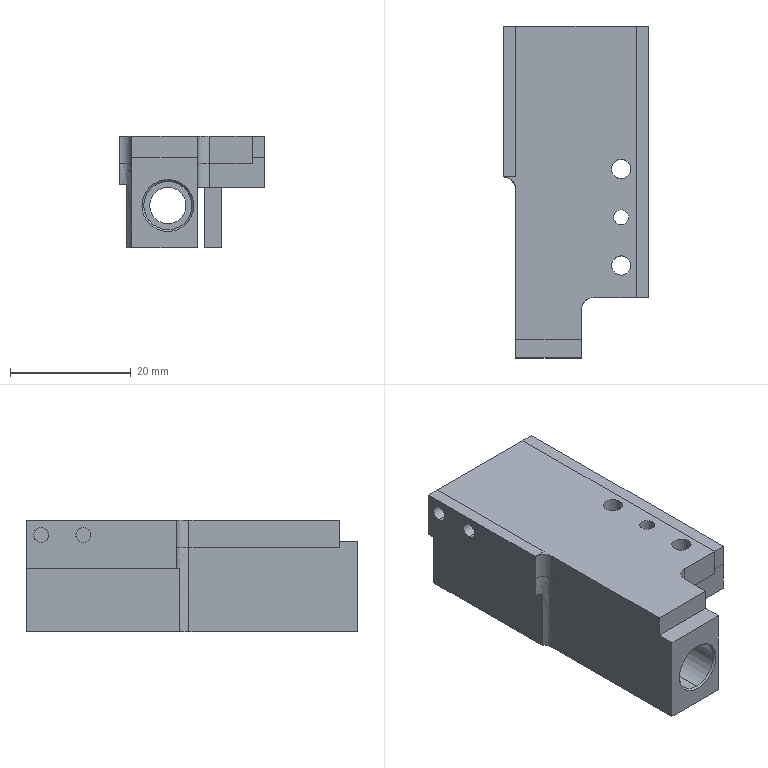NC program | NX | posted with a generic post | part box 24.15 x 55 x 18.5 mm
Lines 1 to 546 of 2247:
N10 G17 G21 G94 G90
(FLOOR_WALL , TOOL : D63)
N12 T01 M6
N14 G54
N16 G17 G0 G90 X67. Y0. B0. C0. S6500 M3
N18 G43 Z30. H1
N20 Z3.
N22 G94 G1 Z0. F1500.
N24 X64.
N26 X-64.
N28 X-67.
N30 Z3.
N32 G0 Z30.
N34 M5
(DRILLING , TOOL : D6A45)
N36 T07 M6
N38 G54
N40 G17 G0 G90 X12.2 Y7.5 B0. C0. S5000 M3
N42 G43 Z30. H7
N44 G94 G81 G98 Z-1. F250. R3.
N46 X-3.8
N48 X4.2
N50 G80
N52 G0 X4.2 Y7.5 Z30.
N54 M5
(DRILLING_COPY , TOOL : 2.5ZT)
N56 T12 M6
N58 G54
N60 G17 G0 G90 X4.2 Y7.5 B0. C0. S2000 M3
N62 G43 Z30. H12
N64 G94 G83 G98 Z-10.251 F120. Q2. R3.
N66 G80
N68 G0 X4.2 Y7.5 Z30.
N70 M5
(DRILLING_COPY_COPY , TOOL : 3.2ZT)
N72 T13 M6
N74 G54
N76 G17 G0 G90 X12.2 Y7.5 B0. C0. S2000 M3
N78 G43 Z30. H13
N80 G94 G83 G98 Z-10.461 F120. Q2. R3.
N82 X-3.8
N84 G80
N86 G0 X-3.8 Y7.5 Z30.
N88 M5
(ADAPTIVE_MILLING , TOOL : D10)
N90 T10 M6
N92 G54
N94 G17 G0 G90 X-2.563 Y-24.784 B0. C0. S9500 M3
N96 G43 Z30. H10
N98 Z-15.5
N100 G94 G1 Z-18.5 F1000.
N102 X-2.283 Y-24.003 F3000.
N104 X-2.027 Y-23.215
N106 G3 X-2.563 Y-22.137 R1.017
N108 X-5.626 Y-21.376 R8.28
N110 X-15.494 Y-21.093 R111.643
N112 G2 X-29.992 Y-21.056 R887.815
N114 X-34.117 Y-18.283 R5.999
N116 X-36.04 Y-12.654 R13.273
N118 X-36.465 Y-3.921 R71.329
N120 G1 X-36.474 Y-2.546
N122 X-36.48 Y-0.921
N124 X-36.485 Y1.454
N126 X-36.488 Y5.579
N128 Y14.079
N130 X-36.486 Y14.204
N132 G2 X-33.974 Y18.478 R5.768
N134 X-28.533 Y20.541 R12.381
N136 X-20.179 Y21.031 R59.212
N138 G1 X-19.054 Y21.041
N140 X-17.679 Y21.049
N142 X-15.929 Y21.055
N144 X-13.304 Y21.06
N146 X-8.554 Y21.062
N148 X29.571 Y21.063
N150 G2 X33.873 Y18.609 R5.7
N152 X35.957 Y13.177 R12.22
N154 X36.458 Y4.7 R59.931
N156 G1 X36.467 Y3.7
N158 X36.475 Y2.325
N160 X36.481 Y0.575
N162 X36.485 Y-1.925
N164 X36.488 Y-6.55
N166 Y-14.05
N168 G2 X34.107 Y-18.39 R5.638
N170 X28.571 Y-20.538 R12.149
N172 X19.843 Y-21.034 R61.355
N174 X0.344 Y-21.035 R958.886
N176 X-5.374 Y-20.44 R637.772
N178 G3 X-17.867 Y-20.106 R166.278
N180 G2 X-27.116 Y-20.063 R498.164
N182 X-32.948 Y-16.21 R7.804
N184 X-35.01 Y-9.706 R16.114
N186 X-35.451 Y-0.347 R81.885
N188 X-35.448 Y11.652 R682.299
N190 X-31.733 Y17.436 R7.719
N192 X-25.378 Y19.549 R15.636
N194 X-15.646 Y20.025 R81.099
N196 G1 X-14.521 Y20.033
N198 X-12.896 Y20.041
N200 X-10.771 Y20.046
N202 X-7.521 Y20.05
N204 X-0.646 Y20.052
N206 X26.354
N208 G2 X32.809 Y16.398 R7.614
N210 X34.963 Y10.058 R15.459
N212 X35.449 Y0.452 R77.317
N214 X35.447 Y-11.672 R652.781
N216 X31.726 Y-17.45 R7.705
N218 X25.367 Y-19.553 R15.684
N220 X15.885 Y-20.023 R79.5
N222 X1.636 Y-20.002 R457.511
N224 G3 X-7.714 Y-19.325 R712.588
N226 X-24.461 Y-19.088 R487.014
N228 G2 X-30.768 Y-16.003 R8.647
N230 X-32.273 Y-14.03 R5.197
N232 X-34.106 Y-6.542 R21.984
N234 X-34.454 Y5.074 R140.599
N236 X-34.382 Y9.821 R51.129
N238 X-31.544 Y15.193 R8.556
N240 X-29.567 Y16.793 R5.107
N242 X-22.215 Y18.652 R21.372
N244 X-11.725 Y19.021 R120.261
N246 G1 X-9.975 Y19.029
N248 X-7.85 Y19.035
N250 X-4.6 Y19.039
N252 X1.9 Y19.041
N254 X23.775 Y19.042
N256 X24.15 Y19.037
N258 G2 X31.898 Y14.354 R8.896
N260 X33.963 Y7.584 R17.834
N262 X34.442 Y-3.149 R95.578
N264 X34.404 Y-9.647 R101.765
N266 X29.736 Y-16.498 R8.901
N268 X22.712 Y-18.576 R18.511
N270 X12.476 Y-19.014 R98.538
N272 X1.353 Y-18.92 R191.154
N274 G3 X-21.376 Y-18.122 R270.713
N276 G2 X-26.261 Y-17.241 R12.147
N278 X-28.897 Y-17.023 R12.671
N280 X-30.824 Y-15.96 R5.411
N282 G1 X-31.01 Y-15.817
N284 X-31.184 Y-15.661
N286 X-31.918 Y-14.705
N288 X-31.987 Y-14.586
N290 G2 X-32.662 Y-11.665 R6.267
N292 X-33.33 Y-1.565 R193.716
N294 X-33.384 Y7.558 R133.844
N296 X-32.676 Y10.59 R10.907
N298 G1 X-32.653 Y10.713
N300 X-32.65 Y10.737
N302 Y12.04
N304 X-32.645 Y12.109
N306 G2 X-31.918 Y14.705 R5.901
N308 G1 X-31.537 Y15.201
N310 G3 X-33.509 Y15.923 R-1.1
N312 G1 X-34.849 Y-11.987
N314 G3 X-32.65 Y-12.04 R-1.1
N316 G1 Y10.835
N318 G2 X-32.448 Y13.472 R10.948
N320 X-30.011 Y16.562 R5.458
N322 X-27.09 Y17.235 R6.219
N324 X-17.114 Y17.9 R201.546
N326 X4.259 Y18.03 R887.262
N328 G1 X21.384 Y18.031
N330 X21.634 Y18.03
N332 X22.009 Y18.024
N334 X22.134 Y18.021
N336 X22.384 Y18.012
N338 G2 X30.924 Y12.597 R9.801
N340 X32.948 Y5.55 R19.964
N342 X33.424 Y-4.934 R97.447
N344 X33.038 Y-9.524 R15.823
N346 G1 X32.967 Y-9.764
N348 X32.928 Y-9.883
N350 X32.889 Y-10.002
N352 X32.847 Y-10.119
N354 X32.805 Y-10.237
N356 X32.761 Y-10.354
N358 X32.715 Y-10.471
N360 X32.668 Y-10.586
N362 X32.619 Y-10.701
N364 X32.569 Y-10.816
N366 X32.531 Y-10.935
N368 X32.523 Y-10.962
N370 G2 X30.411 Y-14.24 R5.141
N372 X22.951 Y-17.256 R16.944
N374 X13.237 Y-17.966 R62.382
N376 X-3.501 Y-17.582 R164.578
N378 G3 X-12.757 Y-17.225 R323.497
N380 G1 X-26.382
N382 G3 X-27.288 Y-17.801 R1.011
N384 G1 X-28.004 Y-19.668 Z-18.4
N386 G2 X-28.371 Y-20.309 R1.46
N388 X-29.564 Y-20.407 R1.007
N390 G1 X-32.73 Y-18.414
N392 G2 X-33.721 Y-17.666 R6.355
N394 X-34.708 Y-16.099 R5.08
N396 X-35.323 Y-14.343 R10.431
N398 G1 X-35.432 Y-13.734
N400 X-35.497 Y-13.119
N402 X-36.558 Y5.316
N404 G2 X-35.677 Y13.217 R23.832
N406 G1 X-35.35 Y14.362
N408 X-35.008 Y15.501
N410 G2 X-32.901 Y18.284 R5.916
N412 G1 X-31.237 Y19.475
N414 G2 X-29.922 Y19.344 R1.009
N416 G1 X-28.489 Y17.948 Z-18.5
N418 X-27.919 Y17.41
N420 G3 X-27.34 Y17.225 R1.046
N422 G1 X17.465
N424 X17.784 Y17.204
N426 G2 X22.515 Y16.833 R36.188
N428 X29.919 Y11.03 R10.59
N430 X31.948 Y3.594 R21.625
N432 G3 X32.484 Y2.164 R25.143
N434 G1 X32.645 Y0.934
N436 X32.65 Y0.865
N438 Y-9.965
N440 X32.645 Y-10.034
N442 X32.515 Y-11.026
N444 G3 X34.466 Y-11.443 R1.001
N446 G1 X35.143 Y-9.56 Z-18.4
N448 X35.638 Y-8.182
N450 X35.678 Y-8.015
N452 X35.697 Y-7.844
N454 X35.704 Y-3.679
N456 X35.683 Y0.487
N458 G3 X34.76 Y6.553 R27.751
N460 X33.283 Y10.963 R31.517
N462 X30.819 Y15.312 R23.667
N464 X28.501 Y17.616 R12.703
N466 X25.792 Y19.1 R8.867
N468 G1 X24.902 Y19.388
N470 X23.999 Y19.632
N472 X20.716 Y20.402
N474 G3 X20.092 Y20.347 R1.043
N476 G1 X18.445 Y19.637
N478 X17.142 Y19.064 Z-18.471
N480 G3 X16.762 Y18.642 Z-18.5 R1.053
N482 X17.534 Y17.22 R1.003
N484 G2 X19.834 Y16.674 R6.697
N486 X24.753 Y14.567 R17.133
N488 X29.759 Y7.582 R13.376
N490 G1 X29.837 Y7.344
N492 X29.876 Y7.225
N494 X29.95 Y6.987
N496 X29.986 Y6.867
N498 X30.09 Y6.507
N500 X30.158 Y6.266
N502 X30.257 Y5.904
N504 X30.324 Y5.664
N506 X30.393 Y5.423
N508 X30.43 Y5.304
N510 X30.481 Y5.189
N512 G3 X31.184 Y4.486 R2.923
N514 G2 X32.035 Y3.295 R7.625
N516 G3 X33.915 Y3.385 R1.001
N518 X33.904 Y4.054 Z-18.466 R1.278
N520 G1 X33.652 Y5.352 Z-18.4
N522 X33.199 Y7.642
N524 X32.846 Y8.707
N526 X32.445 Y9.756
N528 X32.117 Y10.426
N530 X31.748 Y11.075
N532 X31.028 Y12.231
N534 X30.264 Y13.359
N536 G3 X26.21 Y17.381 R19.365
N538 G1 X25.473 Y17.863
N540 X24.709 Y18.302
N542 X23.859 Y18.758
N544 X22.996 Y19.192
N546 X22.766 Y19.237
N548 X22.531 Y19.235
N550 X20.745 Y18.976
N552 X19.341 Y18.762 Z-18.471
N554 G3 X18.863 Y18.449 Z-18.5 R1.052
N556 X19.244 Y16.879 R1.003
N558 G2 X20.933 Y15.897 R5.337
N560 X25.413 Y12.323 R21.548
N562 X28.596 Y6.981 R18.553
N564 G3 X29.356 Y5.702 R3.704
N566 G1 X30.13 Y5.318
N568 X30.824 Y4.785
N570 G3 X32.549 Y5.969 R1.101
N572 X32.122 Y6.604 Z-18.461 R1.639
N574 G1 X31.302 Y7.515 Z-18.4
N576 X24.482 Y15.09
N578 X23.144 Y16.576 Z-18.5
N580 X22.113 Y17.721
N582 G3 X20.626 Y16.112 R-1.1
N584 G2 X21.796 Y14.87 R4.553
N586 X25.343 Y10.513 R40.15
N588 G1 X25.479 Y10.303
N590 X25.547 Y10.198
N592 X25.679 Y9.986
N594 X25.81 Y9.773
N596 X25.938 Y9.558
N598 X26.128 Y9.235
N600 X26.314 Y8.909
N602 X26.498 Y8.583
N604 X26.864 Y7.928
N606 X26.925 Y7.819
N608 X27.111 Y7.493
N610 X27.174 Y7.386
N612 X27.239 Y7.278
N614 X27.304 Y7.171
N616 X27.37 Y7.066
N618 X27.437 Y6.96
N620 X27.506 Y6.856
N622 X27.577 Y6.753
N624 G3 X28.897 Y5.848 R1.639
N626 G1 X29.59 Y5.561
N628 G3 X31.049 Y6.213 R1.104
N630 X30.801 Y7.349 Z-18.439 R1.126
N632 G1 X30.308 Y7.95 Z-18.4
N634 X24.5 Y15.04
N636 X23.923 Y15.754 Z-18.446
N638 X23.328 Y16.452 Z-18.492
N640 X23.199 Y16.553 Z-18.5
N642 G3 X21.717 Y14.967 R1.1
N644 G2 X22.38 Y13.667 R5.051
N646 G3 X26.204 Y7.218 R114.868
N648 X27.353 Y6.096 R3.119
N650 G1 X27.471 Y6.058
N652 X27.529 Y6.046
N654 X28.65 Y5.899
N656 G3 X29.81 Y6.569 R1.108
N658 X29.615 Y7.726 Z-18.438 R1.125
N660 G1 X29.156 Y8.338 Z-18.4
N662 X24.89 Y14.016
N664 X24.484 Y14.561 Z-18.434
N666 X24.064 Y15.095 Z-18.468
N668 G3 X23.507 Y15.392 Z-18.5 R1.151
N670 X22.274 Y13.893 R1.102
N672 G2 X22.646 Y12.48 R6.204
N674 G3 X25.633 Y6.753 R16.816
N676 X26.736 Y6.05 R1.822
N678 G1 X27.465
N680 X27.534 Y6.045
N682 G3 X28.605 Y6.681 R1.108
N684 X28.472 Y7.829 Z-18.439 R1.127
N686 G1 X28.041 Y8.486 Z-18.4
N688 X25.04 Y13.055
N690 X24.738 Y13.523 Z-18.428
N692 X24.418 Y13.978 Z-18.456
N694 G3 X23.632 Y14.334 Z-18.5 R1.128
N696 X22.516 Y13.091 R1.103
N698 X22.788 Y10.801 R57.146
N700 X25.096 Y6.438 R9.009
N702 X25.873 Y6.05 R1.407
N704 G1 X26.748
N706 G3 X27.672 Y7.747 R1.102
N708 G1 X24.674 Y12.387
N710 G3 X22.65 Y11.79 R1.101
N712 X22.858 Y9.061 R9.286
N714 X24.591 Y6.228 R5.457
N716 X25.105 Y6.05 R3.353
N718 G1 X25.98
N720 G3 X26.877 Y7.787 R1.101
N722 G1 X24.647 Y10.927
N724 G3 X22.65 Y10.29 R1.101
N726 X22.889 Y7.819 R6.884
N728 X24.118 Y6.143 R2.912
N730 X25.23 Y6.05 R3.098
N732 X26.096 Y7.828 R1.101
N734 G1 X24.616 Y9.718
N736 G3 X22.65 Y9.04 R1.101
N738 X22.867 Y7.07 R4.833
N740 X24.521 Y6.05 R1.462
N742 X25.352 Y7.87 R1.101
N744 G1 X24.913 Y8.386
N746 X24.455 Y8.885
N748 G3 X22.65 Y8.04 R1.101
N750 X22.938 Y6.475 R2.513
N752 X24.097 Y6.05 R1.284
N754 X24.427 Y8.627 R1.311
N756 X22.65 Y7.29 R1.394
N758 X23.838 Y6.05 R1.1
N760 X24.671 Y6.498 R1.014
N762 G1 X24.924 Y6.879
N764 X26.028 Y8.546 Z-18.4
N766 X26.198 Y8.801
N768 X26.409 Y9.024
N770 G2 X27.019 Y9.232 R1.041
N772 G1 X27.642
N774 X28.262 Y9.184
N776 X28.865 Y9.041
N778 X31.04 Y8.333
N780 G2 X34.023 Y6.2 R7.046
N782 X35.385 Y3.233 R7.069
N784 X35.655 Y0.763 R14.725
N786 G1 X35.738 Y-3.075
N788 X35.804 Y-6.914
N790 G2 X35.637 Y-10.366 R39.668
N792 G1 X35.433 Y-12.519
N794 G2 X34.336 Y-13.427 R1.023
N796 G1 X32.337 Y-13.465 Z-18.5
N798 X31.518 Y-13.493
N800 X31.292 Y-13.566
N802 X31.086 Y-13.684
N804 G2 X27.904 Y-15.146 R5.68
N806 X13.67 Y-16.907 R61.934
N808 X-0.324 Y-16.756 R160.432
N810 G1 X-0.447 Y-16.777
N812 X-0.478 Y-16.783
N814 X-1.253 Y-17.065
N816 X-1.372 Y-17.093
N818 X-2.468 Y-17.221
N820 X-2.53 Y-17.225
N822 X-12.78
N824 G3 X-12.72 Y-19.423 R-1.1
N826 G1 X-0.682 Y-18.773
N828 X1.315 Y-18.666 Z-18.4
N830 X20.161 Y-17.648
N832 X22.158 Y-17.54 Z-18.5
N834 X28.967 Y-17.173
N836 G3 X28.764 Y-14.984 R-1.1
N838 G2 X25.215 Y-15.15 R17.986
N840 G1 X25.09 Y-15.153
N842 X24.84 Y-15.164
N844 X24.466 Y-15.183
N846 X24.092 Y-15.206
N848 X23.718 Y-15.232
N850 X23.344 Y-15.262
N852 X22.97 Y-15.293
N854 X21.725 Y-15.401
N856 X20.977 Y-15.462
N858 X20.105 Y-15.53
N860 X19.232 Y-15.595
N862 X18.359 Y-15.657
N864 X17.736 Y-15.695
N866 X17.236 Y-15.724
N868 X16.612 Y-15.755
N870 G2 X1.492 Y-15.836 R189.635
N872 G3 X0.76 Y-16.054 R1.375
N874 G2 X-0.48 Y-16.784 R5.827
N876 G3 X-0.891 Y-18.586 R1.102
N878 X0.155 Y-18.903 Z-18.443 R1.216
N880 G1 X1.016 Y-18.85 Z-18.4
N882 X20.435 Y-17.648
N884 X22.431 Y-17.524 Z-18.5
N886 X25.283 Y-17.348
N888 G3 X25.215 Y-15.15 R1.1
N890 G1 X2.34
N892 X2.215 Y-15.157
N894 X2.091 Y-15.167
N896 G3 X1.318 Y-15.483 R1.362
N898 G1 X0.854 Y-15.975
N900 X0.76 Y-16.054
N902 G3 X2.122 Y-17.78 R1.1
N904 G1 X2.63 Y-17.409
N906 X3.125 Y-17.021
N908 G3 X2.34 Y-15.15 R1.101
N910 X1.445 Y-15.381 R1.285
N912 X1.249 Y-16.743 R1.015
N914 G1 X2.185 Y-18.093
N916 Z-15.5
N918 G0 Z30.
(ZLEVEL_PROFILE , TOOL : D10)
N920 X-29.122 Y18.884
N922 Z-17.
N924 G1 Z-18.5 F1500.
N926 X-28.366 Y17.575
N928 G3 X-27.5 Y17.075 R1.
N930 G1 X17.5
N932 G2 X22.5 Y12.075 R5.
N934 G1 Y5.9
N936 X27.5
N938 G2 X32.5 Y0.9 R5.
N940 G1 Y-10.
N942 G2 X27.5 Y-15. R5.
N944 G1 X1.557
N946 G2 X-2.499 Y-17.075 R5.
N948 G1 X-27.5
N950 G2 X-32.5 Y-12.075 R5.
N952 G1 Y12.075
N954 G2 X-27.5 Y17.075 R5.
N956 G3 X-26.634 Y17.575 R1.
N958 G1 X-25.768 Y19.075
N960 Z-17.
N962 G0 Z30.
(FLOOR_WALL_1_COPY_1 , TOOL : D10)
N964 X30.505 Y7.
N966 Z-0.85
N968 G1 X30.1 Y6.766 F1000.
N970 G3 X29.6 Y5.9 R1.
N972 G1 Y-15. F3000.
N974 G3 X30.1 Y-15.866 R1.
N976 G1 X30.505 Y-16.1
N978 G0 Y7. Z-1.7
N980 G1 X30.1 Y6.766 F1000.
N982 G3 X29.6 Y5.9 R1.
N984 G1 Y-15. F3000.
N986 G3 X30.1 Y-15.866 R1.
N988 G1 X30.505 Y-16.1
N990 G0 Y7. Z-2.55
N992 G1 X30.1 Y6.766 F1000.
N994 G3 X29.6 Y5.9 R1.
N996 G1 Y-15. F3000.
N998 G3 X30.1 Y-15.866 R1.
N1000 G1 X30.505 Y-16.1
N1002 G0 Y7. Z-3.4
N1004 G1 X30.1 Y6.766 F1000.
N1006 G3 X29.6 Y5.9 R1.
N1008 G1 Y-15. F3000.
N1010 G3 X30.1 Y-15.866 R1.
N1012 G1 X30.505 Y-16.1
N1014 G0 Z30.
(FLOOR_WALL_1_COPY , TOOL : D10)
N1016 X32.998 Y6.767
N1018 Z-3.5
N1020 G1 X32.997 Y6.766 F1000.
N1022 G3 X32.497 Y5.9 R1.
N1024 G1 Y-15. F1500.
N1026 X30.
N1028 Y5.9
N1030 G2 X30.5 Y6.766 R1.
N1032 G1 X30.732 Y6.9
N1034 X30.232
N1036 X30. Y6.766 F1000.
N1038 G3 X29.5 Y5.9 R1.
N1040 G1 Y-15. F1500.
N1042 G3 X30. Y-15.866 R1.
N1044 G1 X30.232 Y-16.
N1046 G0 Z30.
N1048 M5